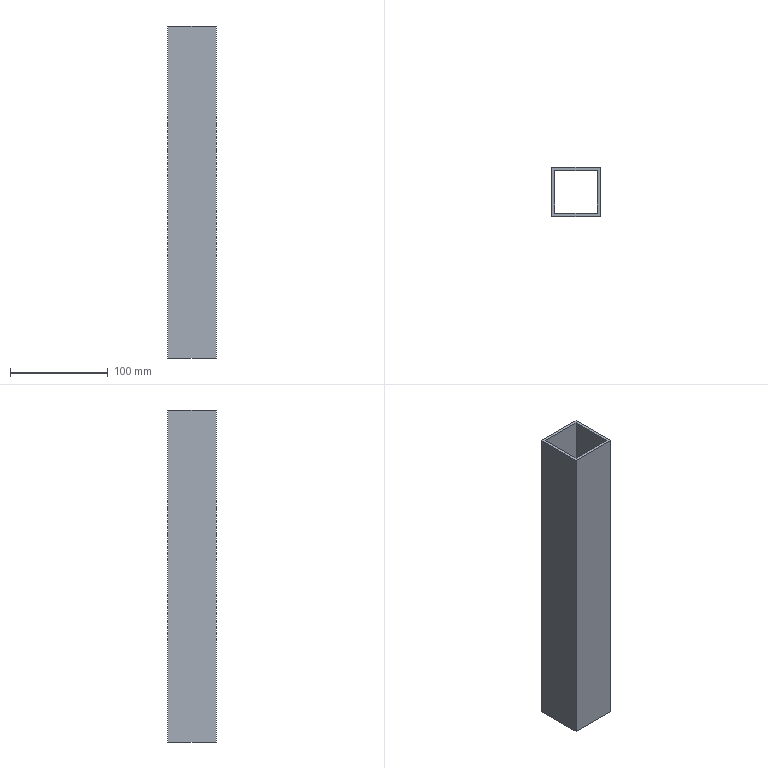Part | SolidWorks | features Extrusion 1 | 1 solid | 10 faces | box 50 x 50 x 340 mm | volume 191760 mm3 | plane 10
STEP:
#1=CARTESIAN_POINT('',(0.,0.,340.));
#2=VERTEX_POINT('',#1);
#3=CARTESIAN_POINT('',(50.,0.,340.));
#4=VERTEX_POINT('',#3);
#5=CARTESIAN_POINT('',(50.,0.,340.));
#6=DIRECTION('',(1.,0.,0.));
#7=VECTOR('',#6,1000.);
#8=LINE('',#5,#7);
#9=EDGE_CURVE('',#2,#4,#8,.T.);
#10=ORIENTED_EDGE('',*,*,#9,.T.);
#11=CARTESIAN_POINT('',(50.,50.,340.));
#12=VERTEX_POINT('',#11);
#13=CARTESIAN_POINT('',(50.,50.,340.));
#14=DIRECTION('',(0.,1.,0.));
#15=VECTOR('',#14,1000.);
#16=LINE('',#13,#15);
#17=EDGE_CURVE('',#4,#12,#16,.T.);
#18=ORIENTED_EDGE('',*,*,#17,.T.);
#19=CARTESIAN_POINT('',(0.,50.,340.));
#20=VERTEX_POINT('',#19);
#21=CARTESIAN_POINT('',(0.,50.,340.));
#22=DIRECTION('',(-1.,0.,0.));
#23=VECTOR('',#22,1000.);
#24=LINE('',#21,#23);
#25=EDGE_CURVE('',#12,#20,#24,.T.);
#26=ORIENTED_EDGE('',*,*,#25,.T.);
#27=CARTESIAN_POINT('',(0.,0.,340.));
#28=DIRECTION('',(0.,-1.,0.));
#29=VECTOR('',#28,1000.);
#30=LINE('',#27,#29);
#31=EDGE_CURVE('',#20,#2,#30,.T.);
#32=ORIENTED_EDGE('',*,*,#31,.T.);
#33=EDGE_LOOP('',(#10,#18,#26,#32));
#34=FACE_OUTER_BOUND('',#33,.T.);
#35=CARTESIAN_POINT('',(3.,3.,340.));
#36=VERTEX_POINT('',#35);
#37=CARTESIAN_POINT('',(47.,3.,340.));
#38=VERTEX_POINT('',#37);
#39=CARTESIAN_POINT('',(47.,3.,340.));
#40=DIRECTION('',(1.,0.,0.));
#41=VECTOR('',#40,1000.);
#42=LINE('',#39,#41);
#43=EDGE_CURVE('',#36,#38,#42,.T.);
#44=ORIENTED_EDGE('',*,*,#43,.F.);
#45=CARTESIAN_POINT('',(3.,47.,340.));
#46=VERTEX_POINT('',#45);
#47=CARTESIAN_POINT('',(3.,3.,340.));
#48=DIRECTION('',(0.,-1.,0.));
#49=VECTOR('',#48,1000.);
#50=LINE('',#47,#49);
#51=EDGE_CURVE('',#46,#36,#50,.T.);
#52=ORIENTED_EDGE('',*,*,#51,.F.);
#53=CARTESIAN_POINT('',(47.,47.,340.));
#54=VERTEX_POINT('',#53);
#55=CARTESIAN_POINT('',(3.,47.,340.));
#56=DIRECTION('',(-1.,0.,0.));
#57=VECTOR('',#56,1000.);
#58=LINE('',#55,#57);
#59=EDGE_CURVE('',#54,#46,#58,.T.);
#60=ORIENTED_EDGE('',*,*,#59,.F.);
#61=CARTESIAN_POINT('',(47.,47.,340.));
#62=DIRECTION('',(0.,1.,0.));
#63=VECTOR('',#62,1000.);
#64=LINE('',#61,#63);
#65=EDGE_CURVE('',#38,#54,#64,.T.);
#66=ORIENTED_EDGE('',*,*,#65,.F.);
#67=EDGE_LOOP('',(#44,#52,#60,#66));
#68=FACE_BOUND('',#67,.T.);
#69=CARTESIAN_POINT('',(0.,0.,340.));
#70=DIRECTION('',(0.,0.,-1.));
#71=DIRECTION('',(-1.,0.,0.));
#72=AXIS2_PLACEMENT_3D('',#69,#70,#71);
#73=PLANE('',#72);
#74=ADVANCED_FACE('',(#34,#68),#73,.F.);
#75=CARTESIAN_POINT('',(0.,0.,0.));
#76=VERTEX_POINT('',#75);
#77=CARTESIAN_POINT('',(50.,0.,0.));
#78=VERTEX_POINT('',#77);
#79=CARTESIAN_POINT('',(50.,0.,0.));
#80=DIRECTION('',(1.,0.,0.));
#81=VECTOR('',#80,1000.);
#82=LINE('',#79,#81);
#83=EDGE_CURVE('',#76,#78,#82,.T.);
#84=ORIENTED_EDGE('',*,*,#83,.F.);
#85=CARTESIAN_POINT('',(0.,50.,0.));
#86=VERTEX_POINT('',#85);
#87=CARTESIAN_POINT('',(0.,0.,0.));
#88=DIRECTION('',(0.,-1.,0.));
#89=VECTOR('',#88,1000.);
#90=LINE('',#87,#89);
#91=EDGE_CURVE('',#86,#76,#90,.T.);
#92=ORIENTED_EDGE('',*,*,#91,.F.);
#93=CARTESIAN_POINT('',(50.,50.,0.));
#94=VERTEX_POINT('',#93);
#95=CARTESIAN_POINT('',(0.,50.,0.));
#96=DIRECTION('',(-1.,0.,0.));
#97=VECTOR('',#96,1000.);
#98=LINE('',#95,#97);
#99=EDGE_CURVE('',#94,#86,#98,.T.);
#100=ORIENTED_EDGE('',*,*,#99,.F.);
#101=CARTESIAN_POINT('',(50.,50.,0.));
#102=DIRECTION('',(0.,1.,0.));
#103=VECTOR('',#102,1000.);
#104=LINE('',#101,#103);
#105=EDGE_CURVE('',#78,#94,#104,.T.);
#106=ORIENTED_EDGE('',*,*,#105,.F.);
#107=EDGE_LOOP('',(#84,#92,#100,#106));
#108=FACE_OUTER_BOUND('',#107,.T.);
#109=CARTESIAN_POINT('',(3.,47.,0.));
#110=VERTEX_POINT('',#109);
#111=CARTESIAN_POINT('',(3.,3.,0.));
#112=VERTEX_POINT('',#111);
#113=CARTESIAN_POINT('',(3.,3.,0.));
#114=DIRECTION('',(0.,-1.,0.));
#115=VECTOR('',#114,1000.);
#116=LINE('',#113,#115);
#117=EDGE_CURVE('',#110,#112,#116,.T.);
#118=ORIENTED_EDGE('',*,*,#117,.T.);
#119=CARTESIAN_POINT('',(47.,3.,0.));
#120=VERTEX_POINT('',#119);
#121=CARTESIAN_POINT('',(47.,3.,0.));
#122=DIRECTION('',(1.,0.,0.));
#123=VECTOR('',#122,1000.);
#124=LINE('',#121,#123);
#125=EDGE_CURVE('',#112,#120,#124,.T.);
#126=ORIENTED_EDGE('',*,*,#125,.T.);
#127=CARTESIAN_POINT('',(47.,47.,0.));
#128=VERTEX_POINT('',#127);
#129=CARTESIAN_POINT('',(47.,47.,0.));
#130=DIRECTION('',(0.,1.,0.));
#131=VECTOR('',#130,1000.);
#132=LINE('',#129,#131);
#133=EDGE_CURVE('',#120,#128,#132,.T.);
#134=ORIENTED_EDGE('',*,*,#133,.T.);
#135=CARTESIAN_POINT('',(3.,47.,0.));
#136=DIRECTION('',(-1.,0.,0.));
#137=VECTOR('',#136,1000.);
#138=LINE('',#135,#137);
#139=EDGE_CURVE('',#128,#110,#138,.T.);
#140=ORIENTED_EDGE('',*,*,#139,.T.);
#141=EDGE_LOOP('',(#118,#126,#134,#140));
#142=FACE_BOUND('',#141,.T.);
#143=CARTESIAN_POINT('',(0.,0.,0.));
#144=DIRECTION('',(0.,0.,-1.));
#145=DIRECTION('',(-1.,0.,0.));
#146=AXIS2_PLACEMENT_3D('',#143,#144,#145);
#147=PLANE('',#146);
#148=ADVANCED_FACE('',(#108,#142),#147,.T.);
#149=ORIENTED_EDGE('',*,*,#83,.T.);
#150=CARTESIAN_POINT('',(50.,0.,340.));
#151=DIRECTION('',(0.,0.,-1.));
#152=VECTOR('',#151,1000.);
#153=LINE('',#150,#152);
#154=EDGE_CURVE('',#4,#78,#153,.T.);
#155=ORIENTED_EDGE('',*,*,#154,.F.);
#156=ORIENTED_EDGE('',*,*,#9,.F.);
#157=CARTESIAN_POINT('',(0.,0.,340.));
#158=DIRECTION('',(0.,0.,-1.));
#159=VECTOR('',#158,1000.);
#160=LINE('',#157,#159);
#161=EDGE_CURVE('',#2,#76,#160,.T.);
#162=ORIENTED_EDGE('',*,*,#161,.T.);
#163=EDGE_LOOP('',(#149,#155,#156,#162));
#164=FACE_OUTER_BOUND('',#163,.T.);
#165=CARTESIAN_POINT('',(50.,0.,340.));
#166=DIRECTION('',(0.,1.,0.));
#167=DIRECTION('',(0.,0.,1.));
#168=AXIS2_PLACEMENT_3D('',#165,#166,#167);
#169=PLANE('',#168);
#170=ADVANCED_FACE('',(#164),#169,.F.);
#171=ORIENTED_EDGE('',*,*,#105,.T.);
#172=CARTESIAN_POINT('',(50.,50.,340.));
#173=DIRECTION('',(0.,0.,-1.));
#174=VECTOR('',#173,1000.);
#175=LINE('',#172,#174);
#176=EDGE_CURVE('',#12,#94,#175,.T.);
#177=ORIENTED_EDGE('',*,*,#176,.F.);
#178=ORIENTED_EDGE('',*,*,#17,.F.);
#179=ORIENTED_EDGE('',*,*,#154,.T.);
#180=EDGE_LOOP('',(#171,#177,#178,#179));
#181=FACE_OUTER_BOUND('',#180,.T.);
#182=CARTESIAN_POINT('',(50.,50.,340.));
#183=DIRECTION('',(-1.,0.,0.));
#184=DIRECTION('',(0.,0.,1.));
#185=AXIS2_PLACEMENT_3D('',#182,#183,#184);
#186=PLANE('',#185);
#187=ADVANCED_FACE('',(#181),#186,.F.);
#188=ORIENTED_EDGE('',*,*,#99,.T.);
#189=CARTESIAN_POINT('',(0.,50.,340.));
#190=DIRECTION('',(0.,0.,-1.));
#191=VECTOR('',#190,1000.);
#192=LINE('',#189,#191);
#193=EDGE_CURVE('',#20,#86,#192,.T.);
#194=ORIENTED_EDGE('',*,*,#193,.F.);
#195=ORIENTED_EDGE('',*,*,#25,.F.);
#196=ORIENTED_EDGE('',*,*,#176,.T.);
#197=EDGE_LOOP('',(#188,#194,#195,#196));
#198=FACE_OUTER_BOUND('',#197,.T.);
#199=CARTESIAN_POINT('',(0.,50.,340.));
#200=DIRECTION('',(0.,-1.,0.));
#201=DIRECTION('',(0.,0.,-1.));
#202=AXIS2_PLACEMENT_3D('',#199,#200,#201);
#203=PLANE('',#202);
#204=ADVANCED_FACE('',(#198),#203,.F.);
#205=ORIENTED_EDGE('',*,*,#91,.T.);
#206=ORIENTED_EDGE('',*,*,#161,.F.);
#207=ORIENTED_EDGE('',*,*,#31,.F.);
#208=ORIENTED_EDGE('',*,*,#193,.T.);
#209=EDGE_LOOP('',(#205,#206,#207,#208));
#210=FACE_OUTER_BOUND('',#209,.T.);
#211=CARTESIAN_POINT('',(0.,0.,340.));
#212=DIRECTION('',(1.,0.,0.));
#213=DIRECTION('',(0.,0.,-1.));
#214=AXIS2_PLACEMENT_3D('',#211,#212,#213);
#215=PLANE('',#214);
#216=ADVANCED_FACE('',(#210),#215,.F.);
#217=ORIENTED_EDGE('',*,*,#125,.F.);
#218=CARTESIAN_POINT('',(3.,3.,340.));
#219=DIRECTION('',(0.,0.,-1.));
#220=VECTOR('',#219,1000.);
#221=LINE('',#218,#220);
#222=EDGE_CURVE('',#36,#112,#221,.T.);
#223=ORIENTED_EDGE('',*,*,#222,.F.);
#224=ORIENTED_EDGE('',*,*,#43,.T.);
#225=CARTESIAN_POINT('',(47.,3.,340.));
#226=DIRECTION('',(0.,0.,-1.));
#227=VECTOR('',#226,1000.);
#228=LINE('',#225,#227);
#229=EDGE_CURVE('',#38,#120,#228,.T.);
#230=ORIENTED_EDGE('',*,*,#229,.T.);
#231=EDGE_LOOP('',(#217,#223,#224,#230));
#232=FACE_OUTER_BOUND('',#231,.T.);
#233=CARTESIAN_POINT('',(47.,3.,340.));
#234=DIRECTION('',(0.,1.,0.));
#235=DIRECTION('',(0.,0.,1.));
#236=AXIS2_PLACEMENT_3D('',#233,#234,#235);
#237=PLANE('',#236);
#238=ADVANCED_FACE('',(#232),#237,.T.);
#239=ORIENTED_EDGE('',*,*,#133,.F.);
#240=ORIENTED_EDGE('',*,*,#229,.F.);
#241=ORIENTED_EDGE('',*,*,#65,.T.);
#242=CARTESIAN_POINT('',(47.,47.,340.));
#243=DIRECTION('',(0.,0.,-1.));
#244=VECTOR('',#243,1000.);
#245=LINE('',#242,#244);
#246=EDGE_CURVE('',#54,#128,#245,.T.);
#247=ORIENTED_EDGE('',*,*,#246,.T.);
#248=EDGE_LOOP('',(#239,#240,#241,#247));
#249=FACE_OUTER_BOUND('',#248,.T.);
#250=CARTESIAN_POINT('',(47.,47.,340.));
#251=DIRECTION('',(-1.,0.,0.));
#252=DIRECTION('',(0.,0.,1.));
#253=AXIS2_PLACEMENT_3D('',#250,#251,#252);
#254=PLANE('',#253);
#255=ADVANCED_FACE('',(#249),#254,.T.);
#256=ORIENTED_EDGE('',*,*,#139,.F.);
#257=ORIENTED_EDGE('',*,*,#246,.F.);
#258=ORIENTED_EDGE('',*,*,#59,.T.);
#259=CARTESIAN_POINT('',(3.,47.,340.));
#260=DIRECTION('',(0.,0.,-1.));
#261=VECTOR('',#260,1000.);
#262=LINE('',#259,#261);
#263=EDGE_CURVE('',#46,#110,#262,.T.);
#264=ORIENTED_EDGE('',*,*,#263,.T.);
#265=EDGE_LOOP('',(#256,#257,#258,#264));
#266=FACE_OUTER_BOUND('',#265,.T.);
#267=CARTESIAN_POINT('',(3.,47.,340.));
#268=DIRECTION('',(0.,-1.,0.));
#269=DIRECTION('',(0.,0.,-1.));
#270=AXIS2_PLACEMENT_3D('',#267,#268,#269);
#271=PLANE('',#270);
#272=ADVANCED_FACE('',(#266),#271,.T.);
#273=ORIENTED_EDGE('',*,*,#117,.F.);
#274=ORIENTED_EDGE('',*,*,#263,.F.);
#275=ORIENTED_EDGE('',*,*,#51,.T.);
#276=ORIENTED_EDGE('',*,*,#222,.T.);
#277=EDGE_LOOP('',(#273,#274,#275,#276));
#278=FACE_OUTER_BOUND('',#277,.T.);
#279=CARTESIAN_POINT('',(3.,3.,340.));
#280=DIRECTION('',(1.,0.,0.));
#281=DIRECTION('',(0.,0.,-1.));
#282=AXIS2_PLACEMENT_3D('',#279,#280,#281);
#283=PLANE('',#282);
#284=ADVANCED_FACE('',(#278),#283,.T.);
#285=CLOSED_SHELL('',(#74,#148,#170,#187,#204,#216,#238,#255,#272,#284));
#286=MANIFOLD_SOLID_BREP('',#285);
#287=CARTESIAN_POINT('',(0.,0.,0.));
#288=DIRECTION('',(0.,0.,1.));
#289=DIRECTION('',(1.,0.,0.));
#290=AXIS2_PLACEMENT_3D('',#287,#288,#289);
#291=(LENGTH_UNIT()NAMED_UNIT(*)SI_UNIT(.MILLI.,.METRE.));
#292=UNCERTAINTY_MEASURE_WITH_UNIT(LENGTH_MEASURE(0.00001),#291,'','');
#293=(NAMED_UNIT(*)PLANE_ANGLE_UNIT()SI_UNIT($,.RADIAN.));
#294=(NAMED_UNIT(*)SI_UNIT($,.STERADIAN.)SOLID_ANGLE_UNIT());
#295=(GEOMETRIC_REPRESENTATION_CONTEXT(3)GLOBAL_UNCERTAINTY_ASSIGNED_CONTEXT((#292))GLOBAL_UNIT_ASSIGNED_CONTEXT((#291,#293,#294))REPRESENTATION_CONTEXT('',''));
#296=ADVANCED_BREP_SHAPE_REPRESENTATION('',(#286,#290),#295);